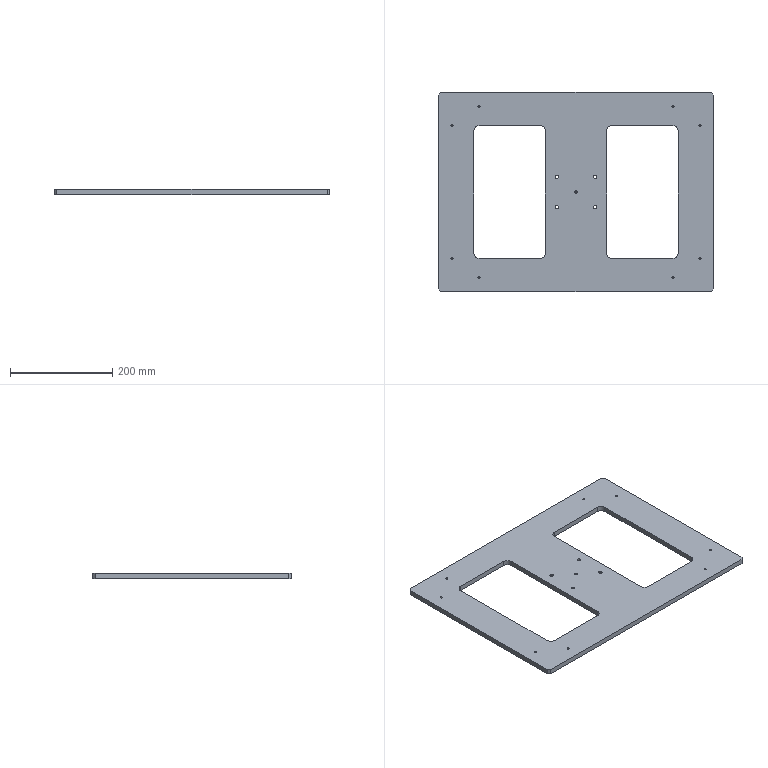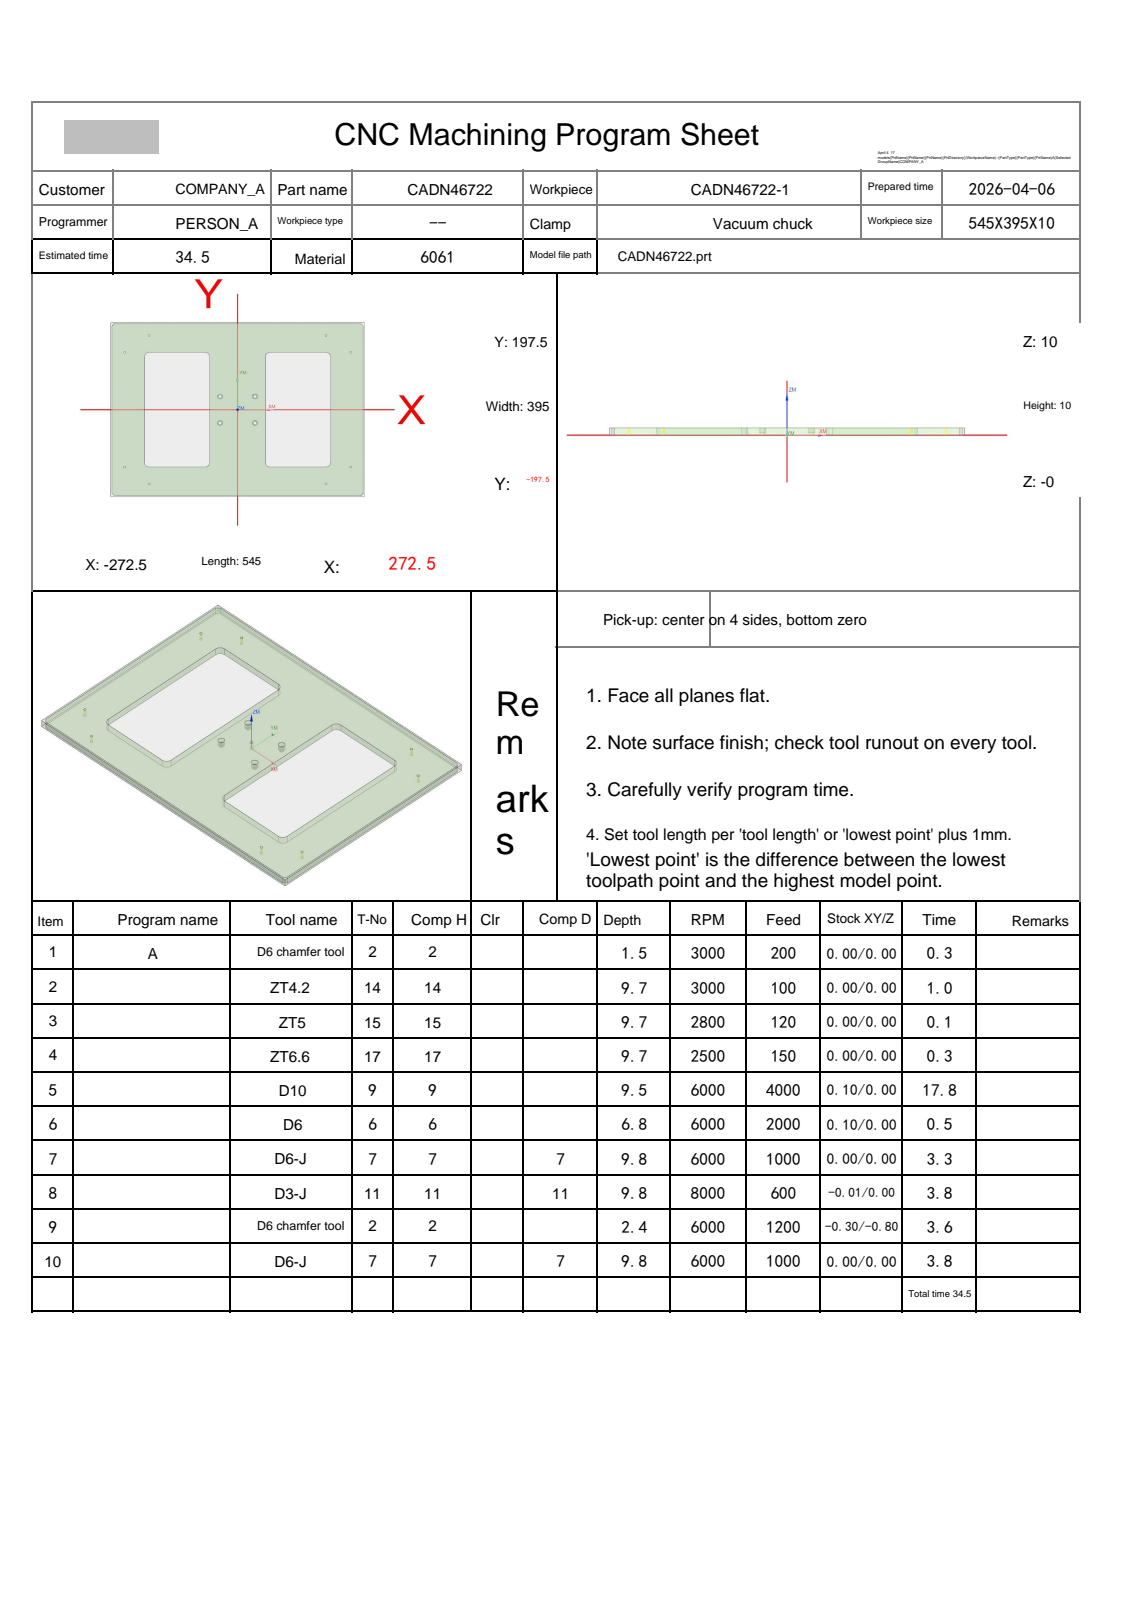NC program | NX | posted by the shop | part box 540 x 390 x 10 mm
Lines 1059 to 1853 of 3473:
N8 T11 M06
(D3-J  D=3. R=0. H=11 ce=0.00 di=0.00)
G00 G90 G54 X190.438 Y-168.3 M03 S8000
G43 H11 Z30.
M08
Z10.5
G01 X190.482 Y-168.239 Z10.496 F600.
X190.533 Y-168.073 Z10.487
Y-167.927 Z10.479
X190.482 Y-167.761 Z10.47
X190.38 Y-167.62 Z10.461
X190.239 Y-167.518 Z10.452
X190.073 Y-167.467 Z10.443
X189.927 Z10.435
X189.761 Y-167.518 Z10.426
X189.62 Y-167.62 Z10.417
X189.518 Y-167.761 Z10.408
X189.467 Y-167.927 Z10.399
Y-168.073 Z10.391
X189.514 Y-168.231 Z10.382
X189.607 Y-168.367 Z10.374
X189.737 Y-168.469 Z10.365
X189.892 Y-168.527 Z10.357
X190.073 Y-168.533 Z10.347
X190.239 Y-168.482 Z10.338
X190.38 Y-168.38 Z10.329
X190.482 Y-168.239 Z10.32
X190.533 Y-168.073 Z10.311
Y-167.927 Z10.303
X190.482 Y-167.761 Z10.294
X190.38 Y-167.62 Z10.285
X190.239 Y-167.518 Z10.276
X190.073 Y-167.467 Z10.267
X189.927 Z10.259
X189.761 Y-167.518 Z10.25
X189.62 Y-167.62 Z10.241
X189.518 Y-167.761 Z10.232
X189.467 Y-167.927 Z10.222
Y-168.073 Z10.215
X189.514 Y-168.231 Z10.206
X189.607 Y-168.367 Z10.197
X189.737 Y-168.469 Z10.189
X189.892 Y-168.527 Z10.18
X190.073 Y-168.533 Z10.171
X190.239 Y-168.482 Z10.162
X190.38 Y-168.38 Z10.152
X190.482 Y-168.239 Z10.143
X190.533 Y-168.073 Z10.134
Y-167.927 Z10.127
X190.482 Y-167.761 Z10.117
X190.38 Y-167.62 Z10.108
X190.239 Y-167.518 Z10.099
X190.073 Y-167.467 Z10.09
X189.927 Z10.082
X189.761 Y-167.518 Z10.073
X189.62 Y-167.62 Z10.064
X189.518 Y-167.761 Z10.055
X189.467 Y-167.927 Z10.046
Y-168.073 Z10.038
X189.514 Y-168.231 Z10.03
X189.607 Y-168.367 Z10.021
X189.737 Y-168.469 Z10.012
X189.892 Y-168.527 Z10.004
X189.965 Y-168.532 Z10.
G41 D11
X190. Y-168.567
G03 X190.567 Y-168. Z9.926 I0.0 J.567
X190. Y-167.433 Z9.852 I-.567 J0.0
X189.433 Y-168. Z9.777 I0.0 J-.567
X190. Y-168.567 Z9.703 I.567 J0.0
X190.567 Y-168. Z9.629 I0.0 J.567
X190. Y-167.433 Z9.555 I-.567 J0.0
X189.433 Y-168. Z9.48 I0.0 J-.567
X190. Y-168.567 Z9.406 I.567 J0.0
X190.567 Y-168. Z9.332 I0.0 J.567
X190. Y-167.433 Z9.258 I-.567 J0.0
X189.433 Y-168. Z9.183 I0.0 J-.567
X190. Y-168.567 Z9.109 I.567 J0.0
X190.567 Y-168. Z9.035 I0.0 J.567
X190. Y-167.433 Z8.961 I-.567 J0.0
X189.433 Y-168. Z8.886 I0.0 J-.567
X190. Y-168.567 Z8.812 I.567 J0.0
X190.567 Y-168. Z8.738 I0.0 J.567
X190. Y-167.433 Z8.664 I-.567 J0.0
X189.433 Y-168. Z8.589 I0.0 J-.567
X190. Y-168.567 Z8.515 I.567 J0.0
X190.567 Y-168. Z8.441 I0.0 J.567
X190. Y-167.433 Z8.367 I-.567 J0.0
X189.433 Y-168. Z8.292 I0.0 J-.567
X190. Y-168.567 Z8.218 I.567 J0.0
X190.567 Y-168. Z8.144 I0.0 J.567
X190. Y-167.433 Z8.07 I-.567 J0.0
X189.433 Y-168. Z7.995 I0.0 J-.567
X190. Y-168.567 Z7.921 I.567 J0.0
X190.567 Y-168. Z7.847 I0.0 J.567
X190. Y-167.433 Z7.773 I-.567 J0.0
X189.433 Y-168. Z7.698 I0.0 J-.567
X190. Y-168.567 Z7.624 I.567 J0.0
X190.567 Y-168. Z7.55 I0.0 J.567
X190. Y-167.433 Z7.476 I-.567 J0.0
X189.433 Y-168. Z7.402 I0.0 J-.567
X190. Y-168.567 Z7.327 I.567 J0.0
X190.567 Y-168. Z7.253 I0.0 J.567
X190. Y-167.433 Z7.179 I-.567 J0.0
X189.433 Y-168. Z7.105 I0.0 J-.567
X190. Y-168.567 Z7.03 I.567 J0.0
X190.567 Y-168. Z6.956 I0.0 J.567
X190. Y-167.433 Z6.882 I-.567 J0.0
X189.433 Y-168. Z6.808 I0.0 J-.567
X190. Y-168.567 Z6.733 I.567 J0.0
X190.567 Y-168. Z6.659 I0.0 J.567
X190. Y-167.433 Z6.585 I-.567 J0.0
X189.433 Y-168. Z6.511 I0.0 J-.567
X190. Y-168.567 Z6.436 I.567 J0.0
X190.567 Y-168. Z6.362 I0.0 J.567
X190. Y-167.433 Z6.288 I-.567 J0.0
X189.433 Y-168. Z6.214 I0.0 J-.567
X190. Y-168.567 Z6.139 I.567 J0.0
X190.567 Y-168. Z6.065 I0.0 J.567
X190. Y-167.433 Z5.991 I-.567 J0.0
X189.433 Y-168. Z5.917 I0.0 J-.567
X190. Y-168.567 Z5.842 I.567 J0.0
X190.567 Y-168. Z5.768 I0.0 J.567
X190. Y-167.433 Z5.694 I-.567 J0.0
X189.433 Y-168. Z5.62 I0.0 J-.567
X190. Y-168.567 Z5.545 I.567 J0.0
X190.567 Y-168. Z5.471 I0.0 J.567
X190. Y-167.433 Z5.397 I-.567 J0.0
X189.433 Y-168. Z5.323 I0.0 J-.567
X190. Y-168.567 Z5.248 I.567 J0.0
X190.567 Y-168. Z5.174 I0.0 J.567
X190. Y-167.433 Z5.1 I-.567 J0.0
X189.433 Y-168. Z5.026 I0.0 J-.567
X190. Y-168.567 Z4.952 I.567 J0.0
X190.567 Y-168. Z4.877 I0.0 J.567
X190. Y-167.433 Z4.803 I-.567 J0.0
X189.433 Y-168. Z4.729 I0.0 J-.567
X190. Y-168.567 Z4.655 I.567 J0.0
X190.567 Y-168. Z4.58 I0.0 J.567
X190. Y-167.433 Z4.506 I-.567 J0.0
X189.433 Y-168. Z4.432 I0.0 J-.567
X190. Y-168.567 Z4.358 I.567 J0.0
X190.567 Y-168. Z4.283 I0.0 J.567
X190. Y-167.433 Z4.209 I-.567 J0.0
X189.433 Y-168. Z4.135 I0.0 J-.567
X190. Y-168.567 Z4.061 I.567 J0.0
X190.567 Y-168. Z3.986 I0.0 J.567
X190. Y-167.433 Z3.912 I-.567 J0.0
X189.433 Y-168. Z3.838 I0.0 J-.567
X190. Y-168.567 Z3.764 I.567 J0.0
X190.567 Y-168. Z3.689 I0.0 J.567
X190. Y-167.433 Z3.615 I-.567 J0.0
X189.433 Y-168. Z3.541 I0.0 J-.567
X190. Y-168.567 Z3.467 I.567 J0.0
X190.567 Y-168. Z3.392 I0.0 J.567
X190. Y-167.433 Z3.318 I-.567 J0.0
X189.433 Y-168. Z3.244 I0.0 J-.567
X190. Y-168.567 Z3.17 I.567 J0.0
X190.567 Y-168. Z3.095 I0.0 J.567
X190. Y-167.433 Z3.021 I-.567 J0.0
X189.433 Y-168. Z2.947 I0.0 J-.567
X190. Y-168.567 Z2.873 I.567 J0.0
X190.567 Y-168. Z2.798 I0.0 J.567
X190. Y-167.433 Z2.724 I-.567 J0.0
X189.433 Y-168. Z2.65 I0.0 J-.567
X190. Y-168.567 Z2.576 I.567 J0.0
X190.567 Y-168. Z2.502 I0.0 J.567
X190. Y-167.433 Z2.427 I-.567 J0.0
X189.433 Y-168. Z2.353 I0.0 J-.567
X190. Y-168.567 Z2.279 I.567 J0.0
X190.567 Y-168. Z2.205 I0.0 J.567
X190. Y-167.433 Z2.13 I-.567 J0.0
X189.433 Y-168. Z2.056 I0.0 J-.567
X190. Y-168.567 Z1.982 I.567 J0.0
X190.567 Y-168. Z1.908 I0.0 J.567
X190. Y-167.433 Z1.833 I-.567 J0.0
X189.433 Y-168. Z1.759 I0.0 J-.567
X190. Y-168.567 Z1.685 I.567 J0.0
X190.567 Y-168. Z1.611 I0.0 J.567
X190. Y-167.433 Z1.536 I-.567 J0.0
X189.433 Y-168. Z1.462 I0.0 J-.567
X190. Y-168.567 Z1.388 I.567 J0.0
X190.567 Y-168. Z1.314 I0.0 J.567
X190. Y-167.433 Z1.239 I-.567 J0.0
X189.433 Y-168. Z1.165 I0.0 J-.567
X190. Y-168.567 Z1.091 I.567 J0.0
X190.567 Y-168. Z1.017 I0.0 J.567
X190. Y-167.433 Z.942 I-.567 J0.0
X189.433 Y-168. Z.868 I0.0 J-.567
X190. Y-168.567 Z.794 I.567 J0.0
X190.567 Y-168. Z.72 I0.0 J.567
X190. Y-167.433 Z.645 I-.567 J0.0
X189.433 Y-168. Z.571 I0.0 J-.567
X190. Y-168.567 Z.497 I.567 J0.0
X190.567 Y-168. Z.423 I0.0 J.567
X190. Y-167.433 Z.348 I-.567 J0.0
X189.433 Y-168. Z.274 I0.0 J-.567
X190. Y-168.567 Z.2 I.567 J0.0
X190.567 Y-168. I0.0 J.567
X190. Y-167.433 I-.567 J0.0
X189.433 Y-168. I0.0 J-.567
X190. Y-168.567 I.567 J0.0
X190.368 Y-168.432 I0.0 J.567
G01 X190.387 Y-168.412
X190.389 Y-168.384
X190.373 Y-168.361
G40 X190.341 Y-168.323
Z1.2
G00 Z30.
X243.3 Y-129.562
Z10.5
G01 X243.239 Y-129.518 Z10.496
X243.073 Y-129.467 Z10.487
X242.927 Z10.479
X242.761 Y-129.518 Z10.47
X242.62 Y-129.62 Z10.461
X242.518 Y-129.761 Z10.452
X242.467 Y-129.927 Z10.443
Y-130.073 Z10.435
X242.518 Y-130.239 Z10.426
X242.62 Y-130.38 Z10.417
X242.761 Y-130.482 Z10.408
X242.927 Y-130.533 Z10.399
X243.073 Z10.391
X243.231 Y-130.486 Z10.382
X243.367 Y-130.393 Z10.374
X243.469 Y-130.263 Z10.365
X243.527 Y-130.108 Z10.357
X243.533 Y-129.927 Z10.347
X243.482 Y-129.761 Z10.338
X243.38 Y-129.62 Z10.329
X243.239 Y-129.518 Z10.32
X243.073 Y-129.467 Z10.311
X242.927 Z10.303
X242.761 Y-129.518 Z10.294
X242.62 Y-129.62 Z10.285
X242.518 Y-129.761 Z10.276
X242.467 Y-129.927 Z10.267
Y-130.073 Z10.259
X242.518 Y-130.239 Z10.25
X242.62 Y-130.38 Z10.241
X242.761 Y-130.482 Z10.232
X242.927 Y-130.533 Z10.222
X243.073 Z10.215
X243.231 Y-130.486 Z10.206
X243.367 Y-130.393 Z10.197
X243.469 Y-130.263 Z10.189
X243.527 Y-130.108 Z10.18
X243.533 Y-129.927 Z10.171
X243.482 Y-129.761 Z10.162
X243.38 Y-129.62 Z10.152
X243.239 Y-129.518 Z10.143
X243.073 Y-129.467 Z10.134
X242.927 Z10.127
X242.761 Y-129.518 Z10.117
X242.62 Y-129.62 Z10.108
X242.518 Y-129.761 Z10.099
X242.467 Y-129.927 Z10.09
Y-130.073 Z10.082
X242.518 Y-130.239 Z10.073
X242.62 Y-130.38 Z10.064
X242.761 Y-130.482 Z10.055
X242.927 Y-130.533 Z10.046
X243.073 Z10.038
X243.231 Y-130.486 Z10.03
X243.367 Y-130.393 Z10.021
X243.469 Y-130.263 Z10.012
X243.527 Y-130.108 Z10.004
X243.532 Y-130.035 Z10.
G41 D11
X243.567 Y-130.
G03 X243. Y-129.433 Z9.926 I-.567 J0.0
X242.433 Y-130. Z9.852 I0.0 J-.567
X243. Y-130.567 Z9.777 I.567 J0.0
X243.567 Y-130. Z9.703 I0.0 J.567
X243. Y-129.433 Z9.629 I-.567 J0.0
X242.433 Y-130. Z9.555 I0.0 J-.567
X243. Y-130.567 Z9.48 I.567 J0.0
X243.567 Y-130. Z9.406 I0.0 J.567
X243. Y-129.433 Z9.332 I-.567 J0.0
X242.433 Y-130. Z9.258 I0.0 J-.567
X243. Y-130.567 Z9.183 I.567 J0.0
X243.567 Y-130. Z9.109 I0.0 J.567
X243. Y-129.433 Z9.035 I-.567 J0.0
X242.433 Y-130. Z8.961 I0.0 J-.567
X243. Y-130.567 Z8.886 I.567 J0.0
X243.567 Y-130. Z8.812 I0.0 J.567
X243. Y-129.433 Z8.738 I-.567 J0.0
X242.433 Y-130. Z8.664 I0.0 J-.567
X243. Y-130.567 Z8.589 I.567 J0.0
X243.567 Y-130. Z8.515 I0.0 J.567
X243. Y-129.433 Z8.441 I-.567 J0.0
X242.433 Y-130. Z8.367 I0.0 J-.567
X243. Y-130.567 Z8.292 I.567 J0.0
X243.567 Y-130. Z8.218 I0.0 J.567
X243. Y-129.433 Z8.144 I-.567 J0.0
X242.433 Y-130. Z8.07 I0.0 J-.567
X243. Y-130.567 Z7.995 I.567 J0.0
X243.567 Y-130. Z7.921 I0.0 J.567
X243. Y-129.433 Z7.847 I-.567 J0.0
X242.433 Y-130. Z7.773 I0.0 J-.567
X243. Y-130.567 Z7.698 I.567 J0.0
X243.567 Y-130. Z7.624 I0.0 J.567
X243. Y-129.433 Z7.55 I-.567 J0.0
X242.433 Y-130. Z7.476 I0.0 J-.567
X243. Y-130.567 Z7.402 I.567 J0.0
X243.567 Y-130. Z7.327 I0.0 J.567
X243. Y-129.433 Z7.253 I-.567 J0.0
X242.433 Y-130. Z7.179 I0.0 J-.567
X243. Y-130.567 Z7.105 I.567 J0.0
X243.567 Y-130. Z7.03 I0.0 J.567
X243. Y-129.433 Z6.956 I-.567 J0.0
X242.433 Y-130. Z6.882 I0.0 J-.567
X243. Y-130.567 Z6.808 I.567 J0.0
X243.567 Y-130. Z6.733 I0.0 J.567
X243. Y-129.433 Z6.659 I-.567 J0.0
X242.433 Y-130. Z6.585 I0.0 J-.567
X243. Y-130.567 Z6.511 I.567 J0.0
X243.567 Y-130. Z6.436 I0.0 J.567
X243. Y-129.433 Z6.362 I-.567 J0.0
X242.433 Y-130. Z6.288 I0.0 J-.567
X243. Y-130.567 Z6.214 I.567 J0.0
X243.567 Y-130. Z6.139 I0.0 J.567
X243. Y-129.433 Z6.065 I-.567 J0.0
X242.433 Y-130. Z5.991 I0.0 J-.567
X243. Y-130.567 Z5.917 I.567 J0.0
X243.567 Y-130. Z5.842 I0.0 J.567
X243. Y-129.433 Z5.768 I-.567 J0.0
X242.433 Y-130. Z5.694 I0.0 J-.567
X243. Y-130.567 Z5.62 I.567 J0.0
X243.567 Y-130. Z5.545 I0.0 J.567
X243. Y-129.433 Z5.471 I-.567 J0.0
X242.433 Y-130. Z5.397 I0.0 J-.567
X243. Y-130.567 Z5.323 I.567 J0.0
X243.567 Y-130. Z5.248 I0.0 J.567
X243. Y-129.433 Z5.174 I-.567 J0.0
X242.433 Y-130. Z5.1 I0.0 J-.567
X243. Y-130.567 Z5.026 I.567 J0.0
X243.567 Y-130. Z4.952 I0.0 J.567
X243. Y-129.433 Z4.877 I-.567 J0.0
X242.433 Y-130. Z4.803 I0.0 J-.567
X243. Y-130.567 Z4.729 I.567 J0.0
X243.567 Y-130. Z4.655 I0.0 J.567
X243. Y-129.433 Z4.58 I-.567 J0.0
X242.433 Y-130. Z4.506 I0.0 J-.567
X243. Y-130.567 Z4.432 I.567 J0.0
X243.567 Y-130. Z4.358 I0.0 J.567
X243. Y-129.433 Z4.283 I-.567 J0.0
X242.433 Y-130. Z4.209 I0.0 J-.567
X243. Y-130.567 Z4.135 I.567 J0.0
X243.567 Y-130. Z4.061 I0.0 J.567
X243. Y-129.433 Z3.986 I-.567 J0.0
X242.433 Y-130. Z3.912 I0.0 J-.567
X243. Y-130.567 Z3.838 I.567 J0.0
X243.567 Y-130. Z3.764 I0.0 J.567
X243. Y-129.433 Z3.689 I-.567 J0.0
X242.433 Y-130. Z3.615 I0.0 J-.567
X243. Y-130.567 Z3.541 I.567 J0.0
X243.567 Y-130. Z3.467 I0.0 J.567
X243. Y-129.433 Z3.392 I-.567 J0.0
X242.433 Y-130. Z3.318 I0.0 J-.567
X243. Y-130.567 Z3.244 I.567 J0.0
X243.567 Y-130. Z3.17 I0.0 J.567
X243. Y-129.433 Z3.095 I-.567 J0.0
X242.433 Y-130. Z3.021 I0.0 J-.567
X243. Y-130.567 Z2.947 I.567 J0.0
X243.567 Y-130. Z2.873 I0.0 J.567
X243. Y-129.433 Z2.798 I-.567 J0.0
X242.433 Y-130. Z2.724 I0.0 J-.567
X243. Y-130.567 Z2.65 I.567 J0.0
X243.567 Y-130. Z2.576 I0.0 J.567
X243. Y-129.433 Z2.502 I-.567 J0.0
X242.433 Y-130. Z2.427 I0.0 J-.567
X243. Y-130.567 Z2.353 I.567 J0.0
X243.567 Y-130. Z2.279 I0.0 J.567
X243. Y-129.433 Z2.205 I-.567 J0.0
X242.433 Y-130. Z2.13 I0.0 J-.567
X243. Y-130.567 Z2.056 I.567 J0.0
X243.567 Y-130. Z1.982 I0.0 J.567
X243. Y-129.433 Z1.908 I-.567 J0.0
X242.433 Y-130. Z1.833 I0.0 J-.567
X243. Y-130.567 Z1.759 I.567 J0.0
X243.567 Y-130. Z1.685 I0.0 J.567
X243. Y-129.433 Z1.611 I-.567 J0.0
X242.433 Y-130. Z1.536 I0.0 J-.567
X243. Y-130.567 Z1.462 I.567 J0.0
X243.567 Y-130. Z1.388 I0.0 J.567
X243. Y-129.433 Z1.314 I-.567 J0.0
X242.433 Y-130. Z1.239 I0.0 J-.567
X243. Y-130.567 Z1.165 I.567 J0.0
X243.567 Y-130. Z1.091 I0.0 J.567
X243. Y-129.433 Z1.017 I-.567 J0.0
X242.433 Y-130. Z.942 I0.0 J-.567
X243. Y-130.567 Z.868 I.567 J0.0
X243.567 Y-130. Z.794 I0.0 J.567
X243. Y-129.433 Z.72 I-.567 J0.0
X242.433 Y-130. Z.645 I0.0 J-.567
X243. Y-130.567 Z.571 I.567 J0.0
X243.567 Y-130. Z.497 I0.0 J.567
X243. Y-129.433 Z.423 I-.567 J0.0
X242.433 Y-130. Z.348 I0.0 J-.567
X243. Y-130.567 Z.274 I.567 J0.0
X243.567 Y-130. Z.2 I0.0 J.567
X243. Y-129.433 I-.567 J0.0
X242.433 Y-130. I0.0 J-.567
X243. Y-130.567 I.567 J0.0
X243.567 Y-130. I0.0 J.567
X243.432 Y-129.632 I-.567 J0.0
G01 X243.412 Y-129.613
X243.384 Y-129.611
X243.361 Y-129.627
G40 X243.323 Y-129.659
Z1.2
G00 Z30.
X243.3 Y130.438
Z10.5
G01 X243.239 Y130.482 Z10.496
X243.073 Y130.533 Z10.487
X242.927 Z10.479
X242.761 Y130.482 Z10.47
X242.62 Y130.38 Z10.461
X242.518 Y130.239 Z10.452
X242.467 Y130.073 Z10.443
Y129.927 Z10.435
X242.518 Y129.761 Z10.426
X242.62 Y129.62 Z10.417
X242.761 Y129.518 Z10.408
X242.927 Y129.467 Z10.399
X243.073 Z10.391
X243.231 Y129.514 Z10.382
X243.367 Y129.607 Z10.374
X243.469 Y129.737 Z10.365
X243.527 Y129.892 Z10.357
X243.533 Y130.073 Z10.347
X243.482 Y130.239 Z10.338
X243.38 Y130.38 Z10.329
X243.239 Y130.482 Z10.32
X243.073 Y130.533 Z10.311
X242.927 Z10.303
X242.761 Y130.482 Z10.294
X242.62 Y130.38 Z10.285
X242.518 Y130.239 Z10.276
X242.467 Y130.073 Z10.267
Y129.927 Z10.259
X242.518 Y129.761 Z10.25
X242.62 Y129.62 Z10.241
X242.761 Y129.518 Z10.232
X242.927 Y129.467 Z10.222
X243.073 Z10.215
X243.231 Y129.514 Z10.206
X243.367 Y129.607 Z10.197
X243.469 Y129.737 Z10.189
X243.527 Y129.892 Z10.18
X243.533 Y130.073 Z10.171
X243.482 Y130.239 Z10.162
X243.38 Y130.38 Z10.152
X243.239 Y130.482 Z10.143
X243.073 Y130.533 Z10.134
X242.927 Z10.127
X242.761 Y130.482 Z10.117
X242.62 Y130.38 Z10.108
X242.518 Y130.239 Z10.099
X242.467 Y130.073 Z10.09
Y129.927 Z10.082
X242.518 Y129.761 Z10.073
X242.62 Y129.62 Z10.064
X242.761 Y129.518 Z10.055
X242.927 Y129.467 Z10.046
X243.073 Z10.038
X243.231 Y129.514 Z10.03
X243.367 Y129.607 Z10.021
X243.469 Y129.737 Z10.012
X243.527 Y129.892 Z10.004
X243.532 Y129.965 Z10.
G41 D11
X243.567 Y130.
G03 X243. Y130.567 Z9.926 I-.567 J0.0
X242.433 Y130. Z9.852 I0.0 J-.567
X243. Y129.433 Z9.777 I.567 J0.0
X243.567 Y130. Z9.703 I0.0 J.567
X243. Y130.567 Z9.629 I-.567 J0.0
X242.433 Y130. Z9.555 I0.0 J-.567
X243. Y129.433 Z9.48 I.567 J0.0
X243.567 Y130. Z9.406 I0.0 J.567
X243. Y130.567 Z9.332 I-.567 J0.0
X242.433 Y130. Z9.258 I0.0 J-.567
X243. Y129.433 Z9.183 I.567 J0.0
X243.567 Y130. Z9.109 I0.0 J.567
X243. Y130.567 Z9.035 I-.567 J0.0
X242.433 Y130. Z8.961 I0.0 J-.567
X243. Y129.433 Z8.886 I.567 J0.0
X243.567 Y130. Z8.812 I0.0 J.567
X243. Y130.567 Z8.738 I-.567 J0.0
X242.433 Y130. Z8.664 I0.0 J-.567
X243. Y129.433 Z8.589 I.567 J0.0
X243.567 Y130. Z8.515 I0.0 J.567
X243. Y130.567 Z8.441 I-.567 J0.0
X242.433 Y130. Z8.367 I0.0 J-.567
X243. Y129.433 Z8.292 I.567 J0.0
X243.567 Y130. Z8.218 I0.0 J.567
X243. Y130.567 Z8.144 I-.567 J0.0
X242.433 Y130. Z8.07 I0.0 J-.567
X243. Y129.433 Z7.995 I.567 J0.0
X243.567 Y130. Z7.921 I0.0 J.567
X243. Y130.567 Z7.847 I-.567 J0.0
X242.433 Y130. Z7.773 I0.0 J-.567
X243. Y129.433 Z7.698 I.567 J0.0
X243.567 Y130. Z7.624 I0.0 J.567
X243. Y130.567 Z7.55 I-.567 J0.0
X242.433 Y130. Z7.476 I0.0 J-.567
X243. Y129.433 Z7.402 I.567 J0.0
X243.567 Y130. Z7.327 I0.0 J.567
X243. Y130.567 Z7.253 I-.567 J0.0
X242.433 Y130. Z7.179 I0.0 J-.567
X243. Y129.433 Z7.105 I.567 J0.0
X243.567 Y130. Z7.03 I0.0 J.567
X243. Y130.567 Z6.956 I-.567 J0.0
X242.433 Y130. Z6.882 I0.0 J-.567
X243. Y129.433 Z6.808 I.567 J0.0
X243.567 Y130. Z6.733 I0.0 J.567
X243. Y130.567 Z6.659 I-.567 J0.0
X242.433 Y130. Z6.585 I0.0 J-.567
X243. Y129.433 Z6.511 I.567 J0.0
X243.567 Y130. Z6.436 I0.0 J.567
X243. Y130.567 Z6.362 I-.567 J0.0
X242.433 Y130. Z6.288 I0.0 J-.567
X243. Y129.433 Z6.214 I.567 J0.0
X243.567 Y130. Z6.139 I0.0 J.567
X243. Y130.567 Z6.065 I-.567 J0.0
X242.433 Y130. Z5.991 I0.0 J-.567
X243. Y129.433 Z5.917 I.567 J0.0
X243.567 Y130. Z5.842 I0.0 J.567
X243. Y130.567 Z5.768 I-.567 J0.0
X242.433 Y130. Z5.694 I0.0 J-.567
X243. Y129.433 Z5.62 I.567 J0.0
X243.567 Y130. Z5.545 I0.0 J.567
X243. Y130.567 Z5.471 I-.567 J0.0
X242.433 Y130. Z5.397 I0.0 J-.567
X243. Y129.433 Z5.323 I.567 J0.0
X243.567 Y130. Z5.248 I0.0 J.567
X243. Y130.567 Z5.174 I-.567 J0.0
X242.433 Y130. Z5.1 I0.0 J-.567
X243. Y129.433 Z5.026 I.567 J0.0
X243.567 Y130. Z4.952 I0.0 J.567
X243. Y130.567 Z4.877 I-.567 J0.0
X242.433 Y130. Z4.803 I0.0 J-.567
X243. Y129.433 Z4.729 I.567 J0.0
X243.567 Y130. Z4.655 I0.0 J.567
X243. Y130.567 Z4.58 I-.567 J0.0
X242.433 Y130. Z4.506 I0.0 J-.567
X243. Y129.433 Z4.432 I.567 J0.0
X243.567 Y130. Z4.358 I0.0 J.567
X243. Y130.567 Z4.283 I-.567 J0.0
X242.433 Y130. Z4.209 I0.0 J-.567
X243. Y129.433 Z4.135 I.567 J0.0
X243.567 Y130. Z4.061 I0.0 J.567
X243. Y130.567 Z3.986 I-.567 J0.0
X242.433 Y130. Z3.912 I0.0 J-.567
X243. Y129.433 Z3.838 I.567 J0.0
X243.567 Y130. Z3.764 I0.0 J.567
X243. Y130.567 Z3.689 I-.567 J0.0
X242.433 Y130. Z3.615 I0.0 J-.567
X243. Y129.433 Z3.541 I.567 J0.0
X243.567 Y130. Z3.467 I0.0 J.567
X243. Y130.567 Z3.392 I-.567 J0.0
X242.433 Y130. Z3.318 I0.0 J-.567
X243. Y129.433 Z3.244 I.567 J0.0
X243.567 Y130. Z3.17 I0.0 J.567
X243. Y130.567 Z3.095 I-.567 J0.0
X242.433 Y130. Z3.021 I0.0 J-.567
X243. Y129.433 Z2.947 I.567 J0.0
X243.567 Y130. Z2.873 I0.0 J.567
X243. Y130.567 Z2.798 I-.567 J0.0
X242.433 Y130. Z2.724 I0.0 J-.567
X243. Y129.433 Z2.65 I.567 J0.0
X243.567 Y130. Z2.576 I0.0 J.567
X243. Y130.567 Z2.502 I-.567 J0.0
X242.433 Y130. Z2.427 I0.0 J-.567
X243. Y129.433 Z2.353 I.567 J0.0
X243.567 Y130. Z2.279 I0.0 J.567
X243. Y130.567 Z2.205 I-.567 J0.0
X242.433 Y130. Z2.13 I0.0 J-.567
X243. Y129.433 Z2.056 I.567 J0.0
X243.567 Y130. Z1.982 I0.0 J.567
X243. Y130.567 Z1.908 I-.567 J0.0
X242.433 Y130. Z1.833 I0.0 J-.567
X243. Y129.433 Z1.759 I.567 J0.0
X243.567 Y130. Z1.685 I0.0 J.567
X243. Y130.567 Z1.611 I-.567 J0.0
X242.433 Y130. Z1.536 I0.0 J-.567
X243. Y129.433 Z1.462 I.567 J0.0
X243.567 Y130. Z1.388 I0.0 J.567
X243. Y130.567 Z1.314 I-.567 J0.0
X242.433 Y130. Z1.239 I0.0 J-.567
X243. Y129.433 Z1.165 I.567 J0.0
X243.567 Y130. Z1.091 I0.0 J.567
X243. Y130.567 Z1.017 I-.567 J0.0
X242.433 Y130. Z.942 I0.0 J-.567
X243. Y129.433 Z.868 I.567 J0.0
X243.567 Y130. Z.794 I0.0 J.567
X243. Y130.567 Z.72 I-.567 J0.0
X242.433 Y130. Z.645 I0.0 J-.567
X243. Y129.433 Z.571 I.567 J0.0
X243.567 Y130. Z.497 I0.0 J.567
X243. Y130.567 Z.423 I-.567 J0.0
X242.433 Y130. Z.348 I0.0 J-.567
X243. Y129.433 Z.274 I.567 J0.0
X243.567 Y130. Z.2 I0.0 J.567
X243. Y130.567 I-.567 J0.0
X242.433 Y130. I0.0 J-.567
X243. Y129.433 I.567 J0.0
X243.567 Y130. I0.0 J.567
X243.432 Y130.368 I-.567 J0.0
G01 X243.412 Y130.387
X243.384 Y130.389
X243.361 Y130.373
G40 X243.323 Y130.341
Z1.2
G00 Z30.
X189.562 Y168.3
Z10.5
G01 X189.518 Y168.239 Z10.496
X189.467 Y168.073 Z10.487
Y167.927 Z10.479
X189.518 Y167.761 Z10.47
X189.62 Y167.62 Z10.461
X189.761 Y167.518 Z10.452
X189.927 Y167.467 Z10.443
X190.073 Z10.435
X190.239 Y167.518 Z10.426
X190.38 Y167.62 Z10.417
X190.482 Y167.761 Z10.408
X190.533 Y167.927 Z10.399
Y168.073 Z10.391
X190.486 Y168.231 Z10.382
X190.393 Y168.367 Z10.374
X190.263 Y168.469 Z10.365
X190.108 Y168.527 Z10.357
X189.927 Y168.533 Z10.347
X189.761 Y168.482 Z10.338
X189.62 Y168.38 Z10.329
X189.518 Y168.239 Z10.32
X189.467 Y168.073 Z10.311
Y167.927 Z10.303
X189.518 Y167.761 Z10.294
X189.62 Y167.62 Z10.285
X189.761 Y167.518 Z10.276
X189.927 Y167.467 Z10.267
X190.073 Z10.259
X190.239 Y167.518 Z10.25
X190.38 Y167.62 Z10.241
X190.482 Y167.761 Z10.232
X190.533 Y167.927 Z10.222
Y168.073 Z10.215
X190.486 Y168.231 Z10.206
X190.393 Y168.367 Z10.197
X190.263 Y168.469 Z10.189
X190.108 Y168.527 Z10.18
X189.927 Y168.533 Z10.171
X189.761 Y168.482 Z10.162
X189.62 Y168.38 Z10.152
X189.518 Y168.239 Z10.143
X189.467 Y168.073 Z10.134
Y167.927 Z10.127
X189.518 Y167.761 Z10.117
X189.62 Y167.62 Z10.108
X189.761 Y167.518 Z10.099
X189.927 Y167.467 Z10.09
X190.073 Z10.082
X190.239 Y167.518 Z10.073
X190.38 Y167.62 Z10.064
X190.482 Y167.761 Z10.055
X190.533 Y167.927 Z10.046
Y168.073 Z10.038
X190.486 Y168.231 Z10.03
X190.393 Y168.367 Z10.021
X190.263 Y168.469 Z10.012
X190.108 Y168.527 Z10.004
X190.035 Y168.532 Z10.
G41 D11
X190. Y168.567
G03 X189.433 Y168. Z9.926 I0.0 J-.567
X190. Y167.433 Z9.852 I.567 J0.0
X190.567 Y168. Z9.777 I0.0 J.567
X190. Y168.567 Z9.703 I-.567 J0.0
X189.433 Y168. Z9.629 I0.0 J-.567
X190. Y167.433 Z9.555 I.567 J0.0
X190.567 Y168. Z9.48 I0.0 J.567
X190. Y168.567 Z9.406 I-.567 J0.0
X189.433 Y168. Z9.332 I0.0 J-.567
X190. Y167.433 Z9.258 I.567 J0.0
X190.567 Y168. Z9.183 I0.0 J.567
X190. Y168.567 Z9.109 I-.567 J0.0
X189.433 Y168. Z9.035 I0.0 J-.567
X190. Y167.433 Z8.961 I.567 J0.0
X190.567 Y168. Z8.886 I0.0 J.567
X190. Y168.567 Z8.812 I-.567 J0.0
X189.433 Y168. Z8.738 I0.0 J-.567
X190. Y167.433 Z8.664 I.567 J0.0
X190.567 Y168. Z8.589 I0.0 J.567
X190. Y168.567 Z8.515 I-.567 J0.0
X189.433 Y168. Z8.441 I0.0 J-.567
X190. Y167.433 Z8.367 I.567 J0.0
X190.567 Y168. Z8.292 I0.0 J.567
X190. Y168.567 Z8.218 I-.567 J0.0
X189.433 Y168. Z8.144 I0.0 J-.567
X190. Y167.433 Z8.07 I.567 J0.0
X190.567 Y168. Z7.995 I0.0 J.567
X190. Y168.567 Z7.921 I-.567 J0.0
X189.433 Y168. Z7.847 I0.0 J-.567
X190. Y167.433 Z7.773 I.567 J0.0
X190.567 Y168. Z7.698 I0.0 J.567
X190. Y168.567 Z7.624 I-.567 J0.0
X189.433 Y168. Z7.55 I0.0 J-.567
X190. Y167.433 Z7.476 I.567 J0.0
X190.567 Y168. Z7.402 I0.0 J.567
X190. Y168.567 Z7.327 I-.567 J0.0
X189.433 Y168. Z7.253 I0.0 J-.567
X190. Y167.433 Z7.179 I.567 J0.0
X190.567 Y168. Z7.105 I0.0 J.567
X190. Y168.567 Z7.03 I-.567 J0.0
X189.433 Y168. Z6.956 I0.0 J-.567
X190. Y167.433 Z6.882 I.567 J0.0
X190.567 Y168. Z6.808 I0.0 J.567
X190. Y168.567 Z6.733 I-.567 J0.0
X189.433 Y168. Z6.659 I0.0 J-.567
X190. Y167.433 Z6.585 I.567 J0.0
X190.567 Y168. Z6.511 I0.0 J.567
X190. Y168.567 Z6.436 I-.567 J0.0
X189.433 Y168. Z6.362 I0.0 J-.567
X190. Y167.433 Z6.288 I.567 J0.0
X190.567 Y168. Z6.214 I0.0 J.567
X190. Y168.567 Z6.139 I-.567 J0.0
X189.433 Y168. Z6.065 I0.0 J-.567
X190. Y167.433 Z5.991 I.567 J0.0
X190.567 Y168. Z5.917 I0.0 J.567
X190. Y168.567 Z5.842 I-.567 J0.0
X189.433 Y168. Z5.768 I0.0 J-.567
X190. Y167.433 Z5.694 I.567 J0.0
X190.567 Y168. Z5.62 I0.0 J.567
X190. Y168.567 Z5.545 I-.567 J0.0
X189.433 Y168. Z5.471 I0.0 J-.567
X190. Y167.433 Z5.397 I.567 J0.0
X190.567 Y168. Z5.323 I0.0 J.567
X190. Y168.567 Z5.248 I-.567 J0.0
X189.433 Y168. Z5.174 I0.0 J-.567
X190. Y167.433 Z5.1 I.567 J0.0
X190.567 Y168. Z5.026 I0.0 J.567
X190. Y168.567 Z4.952 I-.567 J0.0
X189.433 Y168. Z4.877 I0.0 J-.567
X190. Y167.433 Z4.803 I.567 J0.0
X190.567 Y168. Z4.729 I0.0 J.567
X190. Y168.567 Z4.655 I-.567 J0.0
X189.433 Y168. Z4.58 I0.0 J-.567
X190. Y167.433 Z4.506 I.567 J0.0
X190.567 Y168. Z4.432 I0.0 J.567
X190. Y168.567 Z4.358 I-.567 J0.0
X189.433 Y168. Z4.283 I0.0 J-.567
X190. Y167.433 Z4.209 I.567 J0.0
X190.567 Y168. Z4.135 I0.0 J.567
X190. Y168.567 Z4.061 I-.567 J0.0
X189.433 Y168. Z3.986 I0.0 J-.567
X190. Y167.433 Z3.912 I.567 J0.0
X190.567 Y168. Z3.838 I0.0 J.567
X190. Y168.567 Z3.764 I-.567 J0.0
X189.433 Y168. Z3.689 I0.0 J-.567
X190. Y167.433 Z3.615 I.567 J0.0
X190.567 Y168. Z3.541 I0.0 J.567
X190. Y168.567 Z3.467 I-.567 J0.0
X189.433 Y168. Z3.392 I0.0 J-.567
X190. Y167.433 Z3.318 I.567 J0.0
X190.567 Y168. Z3.244 I0.0 J.567
X190. Y168.567 Z3.17 I-.567 J0.0
X189.433 Y168. Z3.095 I0.0 J-.567
X190. Y167.433 Z3.021 I.567 J0.0
X190.567 Y168. Z2.947 I0.0 J.567
X190. Y168.567 Z2.873 I-.567 J0.0
X189.433 Y168. Z2.798 I0.0 J-.567
X190. Y167.433 Z2.724 I.567 J0.0
X190.567 Y168. Z2.65 I0.0 J.567
X190. Y168.567 Z2.576 I-.567 J0.0
X189.433 Y168. Z2.502 I0.0 J-.567
X190. Y167.433 Z2.427 I.567 J0.0
X190.567 Y168. Z2.353 I0.0 J.567
X190. Y168.567 Z2.279 I-.567 J0.0
X189.433 Y168. Z2.205 I0.0 J-.567
X190. Y167.433 Z2.13 I.567 J0.0
X190.567 Y168. Z2.056 I0.0 J.567
X190. Y168.567 Z1.982 I-.567 J0.0
X189.433 Y168. Z1.908 I0.0 J-.567
X190. Y167.433 Z1.833 I.567 J0.0
X190.567 Y168. Z1.759 I0.0 J.567
X190. Y168.567 Z1.685 I-.567 J0.0
X189.433 Y168. Z1.611 I0.0 J-.567
X190. Y167.433 Z1.536 I.567 J0.0